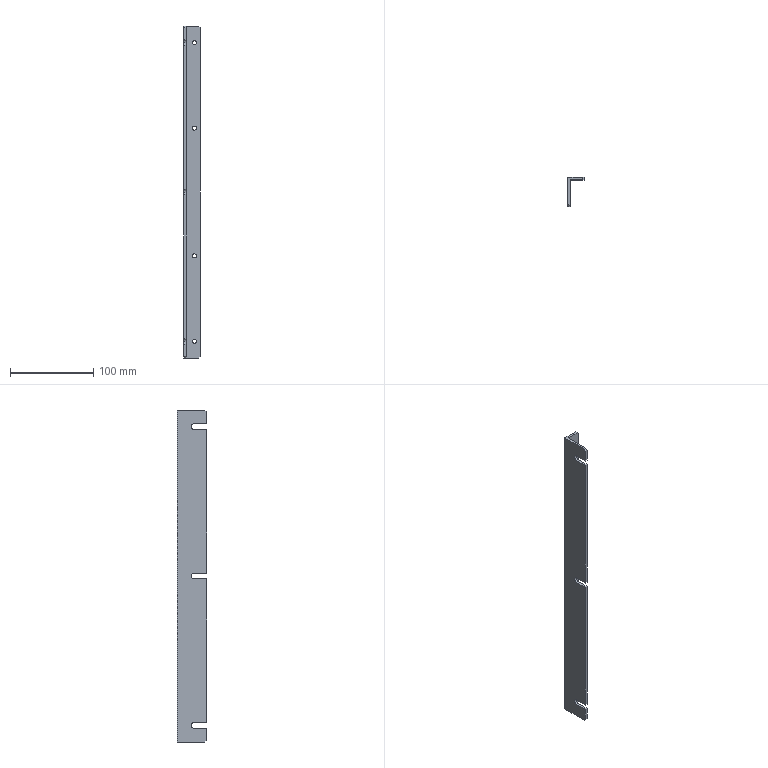Part | SolidWorks | features BaseBody 1 | 1 solid | 35 faces | box 20 x 35 x 400 mm | volume 61095 mm3 | plane 21 | cylinder 14 | commonest cylinder face diameters 5 x8 6.6 x6
STEP:
#1=CARTESIAN_POINT('',(13.,32.,377.5));
#2=VERTEX_POINT('',#1);
#3=CARTESIAN_POINT('',(13.,32.,382.5));
#4=VERTEX_POINT('',#3);
#5=CARTESIAN_POINT('',(13.,32.,380.));
#6=DIRECTION('',(0.,1.,0.));
#7=DIRECTION('',(0.,0.,1.));
#8=AXIS2_PLACEMENT_3D('',#5,#6,#7);
#9=CIRCLE('',#8,2.5);
#10=EDGE_CURVE('',#2,#4,#9,.T.);
#11=ORIENTED_EDGE('',*,*,#10,.F.);
#12=CARTESIAN_POINT('',(13.,35.,377.5));
#13=VERTEX_POINT('',#12);
#14=CARTESIAN_POINT('',(13.,35.,377.5));
#15=DIRECTION('',(0.,1.,0.));
#16=VECTOR('',#15,1000.);
#17=LINE('',#14,#16);
#18=EDGE_CURVE('',#2,#13,#17,.T.);
#19=ORIENTED_EDGE('',*,*,#18,.T.);
#20=CARTESIAN_POINT('',(13.,35.,382.5));
#21=VERTEX_POINT('',#20);
#22=CARTESIAN_POINT('',(13.,35.,380.));
#23=DIRECTION('',(0.,1.,0.));
#24=DIRECTION('',(0.,0.,1.));
#25=AXIS2_PLACEMENT_3D('',#22,#23,#24);
#26=CIRCLE('',#25,2.5);
#27=EDGE_CURVE('',#13,#21,#26,.T.);
#28=ORIENTED_EDGE('',*,*,#27,.T.);
#29=CARTESIAN_POINT('',(13.,35.,382.5));
#30=DIRECTION('',(0.,1.,0.));
#31=VECTOR('',#30,1000.);
#32=LINE('',#29,#31);
#33=EDGE_CURVE('',#4,#21,#32,.T.);
#34=ORIENTED_EDGE('',*,*,#33,.F.);
#35=EDGE_LOOP('',(#11,#19,#28,#34));
#36=FACE_OUTER_BOUND('',#35,.T.);
#37=CARTESIAN_POINT('',(13.,35.,380.));
#38=DIRECTION('',(0.,1.,0.));
#39=DIRECTION('',(0.,0.,1.));
#40=AXIS2_PLACEMENT_3D('',#37,#38,#39);
#41=CYLINDRICAL_SURFACE('',#40,2.5);
#42=ADVANCED_FACE('',(#36),#41,.F.);
#43=CARTESIAN_POINT('',(13.,32.,274.5));
#44=VERTEX_POINT('',#43);
#45=CARTESIAN_POINT('',(13.,32.,279.5));
#46=VERTEX_POINT('',#45);
#47=CARTESIAN_POINT('',(13.,32.,277.));
#48=DIRECTION('',(0.,1.,0.));
#49=DIRECTION('',(0.,0.,1.));
#50=AXIS2_PLACEMENT_3D('',#47,#48,#49);
#51=CIRCLE('',#50,2.5);
#52=EDGE_CURVE('',#44,#46,#51,.T.);
#53=ORIENTED_EDGE('',*,*,#52,.F.);
#54=CARTESIAN_POINT('',(13.,35.,274.5));
#55=VERTEX_POINT('',#54);
#56=CARTESIAN_POINT('',(13.,35.,274.5));
#57=DIRECTION('',(0.,1.,0.));
#58=VECTOR('',#57,1000.);
#59=LINE('',#56,#58);
#60=EDGE_CURVE('',#44,#55,#59,.T.);
#61=ORIENTED_EDGE('',*,*,#60,.T.);
#62=CARTESIAN_POINT('',(13.,35.,279.5));
#63=VERTEX_POINT('',#62);
#64=CARTESIAN_POINT('',(13.,35.,277.));
#65=DIRECTION('',(0.,1.,0.));
#66=DIRECTION('',(0.,0.,1.));
#67=AXIS2_PLACEMENT_3D('',#64,#65,#66);
#68=CIRCLE('',#67,2.5);
#69=EDGE_CURVE('',#55,#63,#68,.T.);
#70=ORIENTED_EDGE('',*,*,#69,.T.);
#71=CARTESIAN_POINT('',(13.,35.,279.5));
#72=DIRECTION('',(0.,1.,0.));
#73=VECTOR('',#72,1000.);
#74=LINE('',#71,#73);
#75=EDGE_CURVE('',#46,#63,#74,.T.);
#76=ORIENTED_EDGE('',*,*,#75,.F.);
#77=EDGE_LOOP('',(#53,#61,#70,#76));
#78=FACE_OUTER_BOUND('',#77,.T.);
#79=CARTESIAN_POINT('',(13.,35.,277.));
#80=DIRECTION('',(0.,1.,0.));
#81=DIRECTION('',(0.,0.,1.));
#82=AXIS2_PLACEMENT_3D('',#79,#80,#81);
#83=CYLINDRICAL_SURFACE('',#82,2.5);
#84=ADVANCED_FACE('',(#78),#83,.F.);
#85=CARTESIAN_POINT('',(13.,32.,120.5));
#86=VERTEX_POINT('',#85);
#87=CARTESIAN_POINT('',(13.,32.,125.5));
#88=VERTEX_POINT('',#87);
#89=CARTESIAN_POINT('',(13.,32.,123.));
#90=DIRECTION('',(0.,1.,0.));
#91=DIRECTION('',(0.,0.,1.));
#92=AXIS2_PLACEMENT_3D('',#89,#90,#91);
#93=CIRCLE('',#92,2.5);
#94=EDGE_CURVE('',#86,#88,#93,.T.);
#95=ORIENTED_EDGE('',*,*,#94,.F.);
#96=CARTESIAN_POINT('',(13.,35.,120.5));
#97=VERTEX_POINT('',#96);
#98=CARTESIAN_POINT('',(13.,35.,120.5));
#99=DIRECTION('',(0.,1.,0.));
#100=VECTOR('',#99,1000.);
#101=LINE('',#98,#100);
#102=EDGE_CURVE('',#86,#97,#101,.T.);
#103=ORIENTED_EDGE('',*,*,#102,.T.);
#104=CARTESIAN_POINT('',(13.,35.,125.5));
#105=VERTEX_POINT('',#104);
#106=CARTESIAN_POINT('',(13.,35.,123.));
#107=DIRECTION('',(0.,1.,0.));
#108=DIRECTION('',(0.,0.,1.));
#109=AXIS2_PLACEMENT_3D('',#106,#107,#108);
#110=CIRCLE('',#109,2.5);
#111=EDGE_CURVE('',#97,#105,#110,.T.);
#112=ORIENTED_EDGE('',*,*,#111,.T.);
#113=CARTESIAN_POINT('',(13.,35.,125.5));
#114=DIRECTION('',(0.,1.,0.));
#115=VECTOR('',#114,1000.);
#116=LINE('',#113,#115);
#117=EDGE_CURVE('',#88,#105,#116,.T.);
#118=ORIENTED_EDGE('',*,*,#117,.F.);
#119=EDGE_LOOP('',(#95,#103,#112,#118));
#120=FACE_OUTER_BOUND('',#119,.T.);
#121=CARTESIAN_POINT('',(13.,35.,123.));
#122=DIRECTION('',(0.,1.,0.));
#123=DIRECTION('',(0.,0.,1.));
#124=AXIS2_PLACEMENT_3D('',#121,#122,#123);
#125=CYLINDRICAL_SURFACE('',#124,2.5);
#126=ADVANCED_FACE('',(#120),#125,.F.);
#127=CARTESIAN_POINT('',(13.,32.,17.5));
#128=VERTEX_POINT('',#127);
#129=CARTESIAN_POINT('',(13.,32.,22.5));
#130=VERTEX_POINT('',#129);
#131=CARTESIAN_POINT('',(13.,32.,20.));
#132=DIRECTION('',(0.,1.,0.));
#133=DIRECTION('',(0.,0.,1.));
#134=AXIS2_PLACEMENT_3D('',#131,#132,#133);
#135=CIRCLE('',#134,2.5);
#136=EDGE_CURVE('',#128,#130,#135,.T.);
#137=ORIENTED_EDGE('',*,*,#136,.F.);
#138=CARTESIAN_POINT('',(13.,35.,17.5));
#139=VERTEX_POINT('',#138);
#140=CARTESIAN_POINT('',(13.,35.,17.5));
#141=DIRECTION('',(0.,1.,0.));
#142=VECTOR('',#141,1000.);
#143=LINE('',#140,#142);
#144=EDGE_CURVE('',#128,#139,#143,.T.);
#145=ORIENTED_EDGE('',*,*,#144,.T.);
#146=CARTESIAN_POINT('',(13.,35.,22.5));
#147=VERTEX_POINT('',#146);
#148=CARTESIAN_POINT('',(13.,35.,20.));
#149=DIRECTION('',(0.,1.,0.));
#150=DIRECTION('',(0.,0.,1.));
#151=AXIS2_PLACEMENT_3D('',#148,#149,#150);
#152=CIRCLE('',#151,2.5);
#153=EDGE_CURVE('',#139,#147,#152,.T.);
#154=ORIENTED_EDGE('',*,*,#153,.T.);
#155=CARTESIAN_POINT('',(13.,35.,22.5));
#156=DIRECTION('',(0.,1.,0.));
#157=VECTOR('',#156,1000.);
#158=LINE('',#155,#157);
#159=EDGE_CURVE('',#130,#147,#158,.T.);
#160=ORIENTED_EDGE('',*,*,#159,.F.);
#161=EDGE_LOOP('',(#137,#145,#154,#160));
#162=FACE_OUTER_BOUND('',#161,.T.);
#163=CARTESIAN_POINT('',(13.,35.,20.));
#164=DIRECTION('',(0.,1.,0.));
#165=DIRECTION('',(0.,0.,1.));
#166=AXIS2_PLACEMENT_3D('',#163,#164,#165);
#167=CYLINDRICAL_SURFACE('',#166,2.5);
#168=ADVANCED_FACE('',(#162),#167,.F.);
#169=CARTESIAN_POINT('',(0.,18.3,20.));
#170=VERTEX_POINT('',#169);
#171=CARTESIAN_POINT('',(0.,15.,23.3));
#172=VERTEX_POINT('',#171);
#173=CARTESIAN_POINT('',(0.,15.,20.));
#174=DIRECTION('',(1.,0.,0.));
#175=DIRECTION('',(0.,1.,0.));
#176=AXIS2_PLACEMENT_3D('',#173,#174,#175);
#177=CIRCLE('',#176,3.3);
#178=EDGE_CURVE('',#170,#172,#177,.T.);
#179=ORIENTED_EDGE('',*,*,#178,.F.);
#180=CARTESIAN_POINT('',(3.,18.3,20.));
#181=VERTEX_POINT('',#180);
#182=CARTESIAN_POINT('',(0.,18.3,20.));
#183=DIRECTION('',(1.,0.,0.));
#184=VECTOR('',#183,1000.);
#185=LINE('',#182,#184);
#186=EDGE_CURVE('',#170,#181,#185,.T.);
#187=ORIENTED_EDGE('',*,*,#186,.T.);
#188=CARTESIAN_POINT('',(3.,15.,23.3));
#189=VERTEX_POINT('',#188);
#190=CARTESIAN_POINT('',(3.,15.,20.));
#191=DIRECTION('',(1.,0.,0.));
#192=DIRECTION('',(0.,1.,0.));
#193=AXIS2_PLACEMENT_3D('',#190,#191,#192);
#194=CIRCLE('',#193,3.3);
#195=EDGE_CURVE('',#181,#189,#194,.T.);
#196=ORIENTED_EDGE('',*,*,#195,.T.);
#197=CARTESIAN_POINT('',(0.,15.,23.3));
#198=DIRECTION('',(1.,0.,0.));
#199=VECTOR('',#198,1000.);
#200=LINE('',#197,#199);
#201=EDGE_CURVE('',#172,#189,#200,.T.);
#202=ORIENTED_EDGE('',*,*,#201,.F.);
#203=EDGE_LOOP('',(#179,#187,#196,#202));
#204=FACE_OUTER_BOUND('',#203,.T.);
#205=CARTESIAN_POINT('',(0.,15.,20.));
#206=DIRECTION('',(1.,0.,0.));
#207=DIRECTION('',(0.,1.,0.));
#208=AXIS2_PLACEMENT_3D('',#205,#206,#207);
#209=CYLINDRICAL_SURFACE('',#208,3.3);
#210=ADVANCED_FACE('',(#204),#209,.F.);
#211=CARTESIAN_POINT('',(0.,18.3,380.));
#212=VERTEX_POINT('',#211);
#213=CARTESIAN_POINT('',(0.,15.,383.3));
#214=VERTEX_POINT('',#213);
#215=CARTESIAN_POINT('',(0.,15.,380.));
#216=DIRECTION('',(1.,0.,0.));
#217=DIRECTION('',(0.,1.,0.));
#218=AXIS2_PLACEMENT_3D('',#215,#216,#217);
#219=CIRCLE('',#218,3.3);
#220=EDGE_CURVE('',#212,#214,#219,.T.);
#221=ORIENTED_EDGE('',*,*,#220,.F.);
#222=CARTESIAN_POINT('',(3.,18.3,380.));
#223=VERTEX_POINT('',#222);
#224=CARTESIAN_POINT('',(0.,18.3,380.));
#225=DIRECTION('',(1.,0.,0.));
#226=VECTOR('',#225,1000.);
#227=LINE('',#224,#226);
#228=EDGE_CURVE('',#212,#223,#227,.T.);
#229=ORIENTED_EDGE('',*,*,#228,.T.);
#230=CARTESIAN_POINT('',(3.,15.,383.3));
#231=VERTEX_POINT('',#230);
#232=CARTESIAN_POINT('',(3.,15.,380.));
#233=DIRECTION('',(1.,0.,0.));
#234=DIRECTION('',(0.,1.,0.));
#235=AXIS2_PLACEMENT_3D('',#232,#233,#234);
#236=CIRCLE('',#235,3.3);
#237=EDGE_CURVE('',#223,#231,#236,.T.);
#238=ORIENTED_EDGE('',*,*,#237,.T.);
#239=CARTESIAN_POINT('',(0.,15.,383.3));
#240=DIRECTION('',(1.,0.,0.));
#241=VECTOR('',#240,1000.);
#242=LINE('',#239,#241);
#243=EDGE_CURVE('',#214,#231,#242,.T.);
#244=ORIENTED_EDGE('',*,*,#243,.F.);
#245=EDGE_LOOP('',(#221,#229,#238,#244));
#246=FACE_OUTER_BOUND('',#245,.T.);
#247=CARTESIAN_POINT('',(0.,15.,380.));
#248=DIRECTION('',(1.,0.,0.));
#249=DIRECTION('',(0.,1.,0.));
#250=AXIS2_PLACEMENT_3D('',#247,#248,#249);
#251=CYLINDRICAL_SURFACE('',#250,3.3);
#252=ADVANCED_FACE('',(#246),#251,.F.);
#253=CARTESIAN_POINT('',(0.,18.3,200.));
#254=VERTEX_POINT('',#253);
#255=CARTESIAN_POINT('',(0.,15.,203.3));
#256=VERTEX_POINT('',#255);
#257=CARTESIAN_POINT('',(0.,15.,200.));
#258=DIRECTION('',(1.,0.,0.));
#259=DIRECTION('',(0.,1.,0.));
#260=AXIS2_PLACEMENT_3D('',#257,#258,#259);
#261=CIRCLE('',#260,3.3);
#262=EDGE_CURVE('',#254,#256,#261,.T.);
#263=ORIENTED_EDGE('',*,*,#262,.F.);
#264=CARTESIAN_POINT('',(3.,18.3,200.));
#265=VERTEX_POINT('',#264);
#266=CARTESIAN_POINT('',(0.,18.3,200.));
#267=DIRECTION('',(1.,0.,0.));
#268=VECTOR('',#267,1000.);
#269=LINE('',#266,#268);
#270=EDGE_CURVE('',#254,#265,#269,.T.);
#271=ORIENTED_EDGE('',*,*,#270,.T.);
#272=CARTESIAN_POINT('',(3.,15.,203.3));
#273=VERTEX_POINT('',#272);
#274=CARTESIAN_POINT('',(3.,15.,200.));
#275=DIRECTION('',(1.,0.,0.));
#276=DIRECTION('',(0.,1.,0.));
#277=AXIS2_PLACEMENT_3D('',#274,#275,#276);
#278=CIRCLE('',#277,3.3);
#279=EDGE_CURVE('',#265,#273,#278,.T.);
#280=ORIENTED_EDGE('',*,*,#279,.T.);
#281=CARTESIAN_POINT('',(0.,15.,203.3));
#282=DIRECTION('',(1.,0.,0.));
#283=VECTOR('',#282,1000.);
#284=LINE('',#281,#283);
#285=EDGE_CURVE('',#256,#273,#284,.T.);
#286=ORIENTED_EDGE('',*,*,#285,.F.);
#287=EDGE_LOOP('',(#263,#271,#280,#286));
#288=FACE_OUTER_BOUND('',#287,.T.);
#289=CARTESIAN_POINT('',(0.,15.,200.));
#290=DIRECTION('',(1.,0.,0.));
#291=DIRECTION('',(0.,1.,0.));
#292=AXIS2_PLACEMENT_3D('',#289,#290,#291);
#293=CYLINDRICAL_SURFACE('',#292,3.3);
#294=ADVANCED_FACE('',(#288),#293,.F.);
#295=CARTESIAN_POINT('',(3.,0.,16.7));
#296=VERTEX_POINT('',#295);
#297=CARTESIAN_POINT('',(3.,15.,16.7));
#298=VERTEX_POINT('',#297);
#299=CARTESIAN_POINT('',(3.,0.,16.7));
#300=DIRECTION('',(0.,1.,0.));
#301=VECTOR('',#300,1000.);
#302=LINE('',#299,#301);
#303=EDGE_CURVE('',#296,#298,#302,.T.);
#304=ORIENTED_EDGE('',*,*,#303,.T.);
#305=CARTESIAN_POINT('',(0.,15.,16.7));
#306=VERTEX_POINT('',#305);
#307=CARTESIAN_POINT('',(0.,15.,16.7));
#308=DIRECTION('',(1.,0.,0.));
#309=VECTOR('',#308,1000.);
#310=LINE('',#307,#309);
#311=EDGE_CURVE('',#306,#298,#310,.T.);
#312=ORIENTED_EDGE('',*,*,#311,.F.);
#313=CARTESIAN_POINT('',(0.,0.,16.7));
#314=VERTEX_POINT('',#313);
#315=CARTESIAN_POINT('',(0.,0.,16.7));
#316=DIRECTION('',(0.,1.,0.));
#317=VECTOR('',#316,1000.);
#318=LINE('',#315,#317);
#319=EDGE_CURVE('',#314,#306,#318,.T.);
#320=ORIENTED_EDGE('',*,*,#319,.F.);
#321=CARTESIAN_POINT('',(0.,0.,16.7));
#322=DIRECTION('',(1.,0.,0.));
#323=VECTOR('',#322,1000.);
#324=LINE('',#321,#323);
#325=EDGE_CURVE('',#314,#296,#324,.T.);
#326=ORIENTED_EDGE('',*,*,#325,.T.);
#327=EDGE_LOOP('',(#304,#312,#320,#326));
#328=FACE_OUTER_BOUND('',#327,.T.);
#329=CARTESIAN_POINT('',(0.,0.,16.7));
#330=DIRECTION('',(0.,0.,-1.));
#331=DIRECTION('',(0.,-1.,0.));
#332=AXIS2_PLACEMENT_3D('',#329,#330,#331);
#333=PLANE('',#332);
#334=ADVANCED_FACE('',(#328),#333,.F.);
#335=CARTESIAN_POINT('',(3.,0.,23.3));
#336=VERTEX_POINT('',#335);
#337=CARTESIAN_POINT('',(3.,0.,23.3));
#338=DIRECTION('',(0.,-1.,0.));
#339=VECTOR('',#338,1000.);
#340=LINE('',#337,#339);
#341=EDGE_CURVE('',#189,#336,#340,.T.);
#342=ORIENTED_EDGE('',*,*,#341,.T.);
#343=CARTESIAN_POINT('',(0.,0.,23.3));
#344=VERTEX_POINT('',#343);
#345=CARTESIAN_POINT('',(0.,0.,23.3));
#346=DIRECTION('',(1.,0.,0.));
#347=VECTOR('',#346,1000.);
#348=LINE('',#345,#347);
#349=EDGE_CURVE('',#344,#336,#348,.T.);
#350=ORIENTED_EDGE('',*,*,#349,.F.);
#351=CARTESIAN_POINT('',(0.,0.,23.3));
#352=DIRECTION('',(0.,-1.,0.));
#353=VECTOR('',#352,1000.);
#354=LINE('',#351,#353);
#355=EDGE_CURVE('',#172,#344,#354,.T.);
#356=ORIENTED_EDGE('',*,*,#355,.F.);
#357=ORIENTED_EDGE('',*,*,#201,.T.);
#358=EDGE_LOOP('',(#342,#350,#356,#357));
#359=FACE_OUTER_BOUND('',#358,.T.);
#360=CARTESIAN_POINT('',(0.,0.,23.3));
#361=DIRECTION('',(0.,0.,1.));
#362=DIRECTION('',(0.,-1.,0.));
#363=AXIS2_PLACEMENT_3D('',#360,#361,#362);
#364=PLANE('',#363);
#365=ADVANCED_FACE('',(#359),#364,.F.);
#366=CARTESIAN_POINT('',(3.,0.,376.7));
#367=VERTEX_POINT('',#366);
#368=CARTESIAN_POINT('',(3.,15.,376.7));
#369=VERTEX_POINT('',#368);
#370=CARTESIAN_POINT('',(3.,0.,376.7));
#371=DIRECTION('',(0.,1.,0.));
#372=VECTOR('',#371,1000.);
#373=LINE('',#370,#372);
#374=EDGE_CURVE('',#367,#369,#373,.T.);
#375=ORIENTED_EDGE('',*,*,#374,.T.);
#376=CARTESIAN_POINT('',(0.,15.,376.7));
#377=VERTEX_POINT('',#376);
#378=CARTESIAN_POINT('',(0.,15.,376.7));
#379=DIRECTION('',(1.,0.,0.));
#380=VECTOR('',#379,1000.);
#381=LINE('',#378,#380);
#382=EDGE_CURVE('',#377,#369,#381,.T.);
#383=ORIENTED_EDGE('',*,*,#382,.F.);
#384=CARTESIAN_POINT('',(0.,0.,376.7));
#385=VERTEX_POINT('',#384);
#386=CARTESIAN_POINT('',(0.,0.,376.7));
#387=DIRECTION('',(0.,1.,0.));
#388=VECTOR('',#387,1000.);
#389=LINE('',#386,#388);
#390=EDGE_CURVE('',#385,#377,#389,.T.);
#391=ORIENTED_EDGE('',*,*,#390,.F.);
#392=CARTESIAN_POINT('',(0.,0.,376.7));
#393=DIRECTION('',(1.,0.,0.));
#394=VECTOR('',#393,1000.);
#395=LINE('',#392,#394);
#396=EDGE_CURVE('',#385,#367,#395,.T.);
#397=ORIENTED_EDGE('',*,*,#396,.T.);
#398=EDGE_LOOP('',(#375,#383,#391,#397));
#399=FACE_OUTER_BOUND('',#398,.T.);
#400=CARTESIAN_POINT('',(0.,0.,376.7));
#401=DIRECTION('',(0.,0.,-1.));
#402=DIRECTION('',(0.,-1.,0.));
#403=AXIS2_PLACEMENT_3D('',#400,#401,#402);
#404=PLANE('',#403);
#405=ADVANCED_FACE('',(#399),#404,.F.);
#406=CARTESIAN_POINT('',(3.,0.,383.3));
#407=VERTEX_POINT('',#406);
#408=CARTESIAN_POINT('',(3.,0.,383.3));
#409=DIRECTION('',(0.,-1.,0.));
#410=VECTOR('',#409,1000.);
#411=LINE('',#408,#410);
#412=EDGE_CURVE('',#231,#407,#411,.T.);
#413=ORIENTED_EDGE('',*,*,#412,.T.);
#414=CARTESIAN_POINT('',(0.,0.,383.3));
#415=VERTEX_POINT('',#414);
#416=CARTESIAN_POINT('',(0.,0.,383.3));
#417=DIRECTION('',(1.,0.,0.));
#418=VECTOR('',#417,1000.);
#419=LINE('',#416,#418);
#420=EDGE_CURVE('',#415,#407,#419,.T.);
#421=ORIENTED_EDGE('',*,*,#420,.F.);
#422=CARTESIAN_POINT('',(0.,0.,383.3));
#423=DIRECTION('',(0.,-1.,0.));
#424=VECTOR('',#423,1000.);
#425=LINE('',#422,#424);
#426=EDGE_CURVE('',#214,#415,#425,.T.);
#427=ORIENTED_EDGE('',*,*,#426,.F.);
#428=ORIENTED_EDGE('',*,*,#243,.T.);
#429=EDGE_LOOP('',(#413,#421,#427,#428));
#430=FACE_OUTER_BOUND('',#429,.T.);
#431=CARTESIAN_POINT('',(0.,0.,383.3));
#432=DIRECTION('',(0.,0.,1.));
#433=DIRECTION('',(1.,0.,0.));
#434=AXIS2_PLACEMENT_3D('',#431,#432,#433);
#435=PLANE('',#434);
#436=ADVANCED_FACE('',(#430),#435,.F.);
#437=CARTESIAN_POINT('',(3.,0.,203.3));
#438=VERTEX_POINT('',#437);
#439=CARTESIAN_POINT('',(3.,15.,203.3));
#440=DIRECTION('',(0.,-1.,0.));
#441=VECTOR('',#440,1000.);
#442=LINE('',#439,#441);
#443=EDGE_CURVE('',#273,#438,#442,.T.);
#444=ORIENTED_EDGE('',*,*,#443,.T.);
#445=CARTESIAN_POINT('',(0.,0.,203.3));
#446=VERTEX_POINT('',#445);
#447=CARTESIAN_POINT('',(0.,0.,203.3));
#448=DIRECTION('',(1.,0.,0.));
#449=VECTOR('',#448,1000.);
#450=LINE('',#447,#449);
#451=EDGE_CURVE('',#446,#438,#450,.T.);
#452=ORIENTED_EDGE('',*,*,#451,.F.);
#453=CARTESIAN_POINT('',(0.,15.,203.3));
#454=DIRECTION('',(0.,-1.,0.));
#455=VECTOR('',#454,1000.);
#456=LINE('',#453,#455);
#457=EDGE_CURVE('',#256,#446,#456,.T.);
#458=ORIENTED_EDGE('',*,*,#457,.F.);
#459=ORIENTED_EDGE('',*,*,#285,.T.);
#460=EDGE_LOOP('',(#444,#452,#458,#459));
#461=FACE_OUTER_BOUND('',#460,.T.);
#462=CARTESIAN_POINT('',(0.,15.,203.3));
#463=DIRECTION('',(0.,0.,1.));
#464=DIRECTION('',(1.,0.,0.));
#465=AXIS2_PLACEMENT_3D('',#462,#463,#464);
#466=PLANE('',#465);
#467=ADVANCED_FACE('',(#461),#466,.F.);
#468=CARTESIAN_POINT('',(3.,0.,196.7));
#469=VERTEX_POINT('',#468);
#470=CARTESIAN_POINT('',(3.,15.,196.7));
#471=VERTEX_POINT('',#470);
#472=CARTESIAN_POINT('',(3.,15.,196.7));
#473=DIRECTION('',(0.,1.,0.));
#474=VECTOR('',#473,1000.);
#475=LINE('',#472,#474);
#476=EDGE_CURVE('',#469,#471,#475,.T.);
#477=ORIENTED_EDGE('',*,*,#476,.T.);
#478=CARTESIAN_POINT('',(0.,15.,196.7));
#479=VERTEX_POINT('',#478);
#480=CARTESIAN_POINT('',(0.,15.,196.7));
#481=DIRECTION('',(1.,0.,0.));
#482=VECTOR('',#481,1000.);
#483=LINE('',#480,#482);
#484=EDGE_CURVE('',#479,#471,#483,.T.);
#485=ORIENTED_EDGE('',*,*,#484,.F.);
#486=CARTESIAN_POINT('',(0.,0.,196.7));
#487=VERTEX_POINT('',#486);
#488=CARTESIAN_POINT('',(0.,15.,196.7));
#489=DIRECTION('',(0.,1.,0.));
#490=VECTOR('',#489,1000.);
#491=LINE('',#488,#490);
#492=EDGE_CURVE('',#487,#479,#491,.T.);
#493=ORIENTED_EDGE('',*,*,#492,.F.);
#494=CARTESIAN_POINT('',(0.,0.,196.7));
#495=DIRECTION('',(1.,0.,0.));
#496=VECTOR('',#495,1000.);
#497=LINE('',#494,#496);
#498=EDGE_CURVE('',#487,#469,#497,.T.);
#499=ORIENTED_EDGE('',*,*,#498,.T.);
#500=EDGE_LOOP('',(#477,#485,#493,#499));
#501=FACE_OUTER_BOUND('',#500,.T.);
#502=CARTESIAN_POINT('',(0.,15.,196.7));
#503=DIRECTION('',(0.,0.,-1.));
#504=DIRECTION('',(0.,-1.,0.));
#505=AXIS2_PLACEMENT_3D('',#502,#503,#504);
#506=PLANE('',#505);
#507=ADVANCED_FACE('',(#501),#506,.F.);
#508=CARTESIAN_POINT('',(20.,32.,398.));
#509=VERTEX_POINT('',#508);
#510=CARTESIAN_POINT('',(18.,32.,400.));
#511=VERTEX_POINT('',#510);
#512=CARTESIAN_POINT('',(18.,32.,400.));
#513=DIRECTION('',(-0.7071,0.,0.7071));
#514=VECTOR('',#513,1000.);
#515=LINE('',#512,#514);
#516=EDGE_CURVE('',#509,#511,#515,.T.);
#517=ORIENTED_EDGE('',*,*,#516,.F.);
#518=CARTESIAN_POINT('',(20.,35.,398.));
#519=VERTEX_POINT('',#518);
#520=CARTESIAN_POINT('',(20.,35.,398.));
#521=DIRECTION('',(0.,-1.,0.));
#522=VECTOR('',#521,1000.);
#523=LINE('',#520,#522);
#524=EDGE_CURVE('',#519,#509,#523,.T.);
#525=ORIENTED_EDGE('',*,*,#524,.F.);
#526=CARTESIAN_POINT('',(18.,35.,400.));
#527=VERTEX_POINT('',#526);
#528=CARTESIAN_POINT('',(18.,35.,400.));
#529=DIRECTION('',(0.7071,0.,-0.7071));
#530=VECTOR('',#529,1000.);
#531=LINE('',#528,#530);
#532=EDGE_CURVE('',#527,#519,#531,.T.);
#533=ORIENTED_EDGE('',*,*,#532,.F.);
#534=CARTESIAN_POINT('',(18.,0.,400.));
#535=DIRECTION('',(0.,1.,0.));
#536=VECTOR('',#535,1000.);
#537=LINE('',#534,#536);
#538=EDGE_CURVE('',#511,#527,#537,.T.);
#539=ORIENTED_EDGE('',*,*,#538,.F.);
#540=EDGE_LOOP('',(#517,#525,#533,#539));
#541=FACE_OUTER_BOUND('',#540,.T.);
#542=CARTESIAN_POINT('',(18.,0.,400.));
#543=DIRECTION('',(-0.7071,0.,-0.7071));
#544=DIRECTION('',(-0.7071,0.,0.7071));
#545=AXIS2_PLACEMENT_3D('',#542,#543,#544);
#546=PLANE('',#545);
#547=ADVANCED_FACE('',(#541),#546,.F.);
#548=CARTESIAN_POINT('',(0.,0.,398.));
#549=VERTEX_POINT('',#548);
#550=CARTESIAN_POINT('',(0.,2.,400.));
#551=VERTEX_POINT('',#550);
#552=CARTESIAN_POINT('',(0.,2.,400.));
#553=DIRECTION('',(0.,0.7071,0.7071));
#554=VECTOR('',#553,1000.);
#555=LINE('',#552,#554);
#556=EDGE_CURVE('',#549,#551,#555,.T.);
#557=ORIENTED_EDGE('',*,*,#556,.F.);
#558=CARTESIAN_POINT('',(3.,0.,398.));
#559=VERTEX_POINT('',#558);
#560=CARTESIAN_POINT('',(3.,0.,398.));
#561=DIRECTION('',(-1.,0.,0.));
#562=VECTOR('',#561,1000.);
#563=LINE('',#560,#562);
#564=EDGE_CURVE('',#559,#549,#563,.T.);
#565=ORIENTED_EDGE('',*,*,#564,.F.);
#566=CARTESIAN_POINT('',(3.,2.,400.));
#567=VERTEX_POINT('',#566);
#568=CARTESIAN_POINT('',(3.,2.,400.));
#569=DIRECTION('',(0.,-0.7071,-0.7071));
#570=VECTOR('',#569,1000.);
#571=LINE('',#568,#570);
#572=EDGE_CURVE('',#567,#559,#571,.T.);
#573=ORIENTED_EDGE('',*,*,#572,.F.);
#574=CARTESIAN_POINT('',(0.,2.,400.));
#575=DIRECTION('',(1.,0.,0.));
#576=VECTOR('',#575,1000.);
#577=LINE('',#574,#576);
#578=EDGE_CURVE('',#551,#567,#577,.T.);
#579=ORIENTED_EDGE('',*,*,#578,.F.);
#580=EDGE_LOOP('',(#557,#565,#573,#579));
#581=FACE_OUTER_BOUND('',#580,.T.);
#582=CARTESIAN_POINT('',(0.,2.,400.));
#583=DIRECTION('',(0.,0.7071,-0.7071));
#584=DIRECTION('',(-1.,0.,0.));
#585=AXIS2_PLACEMENT_3D('',#582,#583,#584);
#586=PLANE('',#585);
#587=ADVANCED_FACE('',(#581),#586,.F.);
#588=CARTESIAN_POINT('',(18.,32.,0.));
#589=VERTEX_POINT('',#588);
#590=CARTESIAN_POINT('',(20.,32.,2.));
#591=VERTEX_POINT('',#590);
#592=CARTESIAN_POINT('',(20.,32.,2.));
#593=DIRECTION('',(0.7071,0.,0.7071));
#594=VECTOR('',#593,1000.);
#595=LINE('',#592,#594);
#596=EDGE_CURVE('',#589,#591,#595,.T.);
#597=ORIENTED_EDGE('',*,*,#596,.F.);
#598=CARTESIAN_POINT('',(18.,35.,0.));
#599=VERTEX_POINT('',#598);
#600=CARTESIAN_POINT('',(18.,32.,0.));
#601=DIRECTION('',(0.,-1.,0.));
#602=VECTOR('',#601,1000.);
#603=LINE('',#600,#602);
#604=EDGE_CURVE('',#599,#589,#603,.T.);
#605=ORIENTED_EDGE('',*,*,#604,.F.);
#606=CARTESIAN_POINT('',(20.,35.,2.));
#607=VERTEX_POINT('',#606);
#608=CARTESIAN_POINT('',(20.,35.,2.));
#609=DIRECTION('',(-0.7071,0.,-0.7071));
#610=VECTOR('',#609,1000.);
#611=LINE('',#608,#610);
#612=EDGE_CURVE('',#607,#599,#611,.T.);
#613=ORIENTED_EDGE('',*,*,#612,.F.);
#614=CARTESIAN_POINT('',(20.,35.,2.));
#615=DIRECTION('',(0.,1.,0.));
#616=VECTOR('',#615,1000.);
#617=LINE('',#614,#616);
#618=EDGE_CURVE('',#591,#607,#617,.T.);
#619=ORIENTED_EDGE('',*,*,#618,.F.);
#620=EDGE_LOOP('',(#597,#605,#613,#619));
#621=FACE_OUTER_BOUND('',#620,.T.);
#622=CARTESIAN_POINT('',(20.,35.,2.));
#623=DIRECTION('',(0.7071,0.,-0.7071));
#624=DIRECTION('',(0.,-1.,0.));
#625=AXIS2_PLACEMENT_3D('',#622,#623,#624);
#626=PLANE('',#625);
#627=ADVANCED_FACE('',(#621),#626,.T.);
#628=CARTESIAN_POINT('',(0.,2.,0.));
#629=VERTEX_POINT('',#628);
#630=CARTESIAN_POINT('',(0.,0.,2.));
#631=VERTEX_POINT('',#630);
#632=CARTESIAN_POINT('',(0.,0.,2.));
#633=DIRECTION('',(0.,-0.7071,0.7071));
#634=VECTOR('',#633,1000.);
#635=LINE('',#632,#634);
#636=EDGE_CURVE('',#629,#631,#635,.T.);
#637=ORIENTED_EDGE('',*,*,#636,.F.);
#638=CARTESIAN_POINT('',(3.,2.,0.));
#639=VERTEX_POINT('',#638);
#640=CARTESIAN_POINT('',(0.,2.,0.));
#641=DIRECTION('',(-1.,0.,0.));
#642=VECTOR('',#641,1000.);
#643=LINE('',#640,#642);
#644=EDGE_CURVE('',#639,#629,#643,.T.);
#645=ORIENTED_EDGE('',*,*,#644,.F.);
#646=CARTESIAN_POINT('',(3.,0.,2.));
#647=VERTEX_POINT('',#646);
#648=CARTESIAN_POINT('',(3.,0.,2.));
#649=DIRECTION('',(0.,0.7071,-0.7071));
#650=VECTOR('',#649,1000.);
#651=LINE('',#648,#650);
#652=EDGE_CURVE('',#647,#639,#651,.T.);
#653=ORIENTED_EDGE('',*,*,#652,.F.);
#654=CARTESIAN_POINT('',(3.,0.,2.));
#655=DIRECTION('',(1.,0.,0.));
#656=VECTOR('',#655,1000.);
#657=LINE('',#654,#656);
#658=EDGE_CURVE('',#631,#647,#657,.T.);
#659=ORIENTED_EDGE('',*,*,#658,.F.);
#660=EDGE_LOOP('',(#637,#645,#653,#659));
#661=FACE_OUTER_BOUND('',#660,.T.);
#662=CARTESIAN_POINT('',(3.,0.,2.));
#663=DIRECTION('',(0.,-0.7071,-0.7071));
#664=DIRECTION('',(0.,-0.7071,0.7071));
#665=AXIS2_PLACEMENT_3D('',#662,#663,#664);
#666=PLANE('',#665);
#667=ADVANCED_FACE('',(#661),#666,.T.);
#668=CARTESIAN_POINT('',(3.,32.,0.));
#669=VERTEX_POINT('',#668);
#670=CARTESIAN_POINT('',(3.,32.,0.));
#671=DIRECTION('',(0.,1.,0.));
#672=VECTOR('',#671,1000.);
#673=LINE('',#670,#672);
#674=EDGE_CURVE('',#639,#669,#673,.T.);
#675=ORIENTED_EDGE('',*,*,#674,.F.);
#676=ORIENTED_EDGE('',*,*,#644,.T.);
#677=CARTESIAN_POINT('',(0.,35.,0.));
#678=VERTEX_POINT('',#677);
#679=CARTESIAN_POINT('',(0.,0.,0.));
#680=DIRECTION('',(0.,-1.,0.));
#681=VECTOR('',#680,1000.);
#682=LINE('',#679,#681);
#683=EDGE_CURVE('',#678,#629,#682,.T.);
#684=ORIENTED_EDGE('',*,*,#683,.F.);
#685=CARTESIAN_POINT('',(0.,35.,0.));
#686=DIRECTION('',(-1.,0.,0.));
#687=VECTOR('',#686,1000.);
#688=LINE('',#685,#687);
#689=EDGE_CURVE('',#599,#678,#688,.T.);
#690=ORIENTED_EDGE('',*,*,#689,.F.);
#691=ORIENTED_EDGE('',*,*,#604,.T.);
#692=CARTESIAN_POINT('',(20.,32.,0.));
#693=DIRECTION('',(1.,0.,0.));
#694=VECTOR('',#693,1000.);
#695=LINE('',#692,#694);
#696=EDGE_CURVE('',#669,#589,#695,.T.);
#697=ORIENTED_EDGE('',*,*,#696,.F.);
#698=EDGE_LOOP('',(#675,#676,#684,#690,#691,#697));
#699=FACE_OUTER_BOUND('',#698,.T.);
#700=CARTESIAN_POINT('',(0.,0.,0.));
#701=DIRECTION('',(0.,0.,-1.));
#702=DIRECTION('',(0.,-1.,0.));
#703=AXIS2_PLACEMENT_3D('',#700,#701,#702);
#704=PLANE('',#703);
#705=ADVANCED_FACE('',(#699),#704,.T.);
#706=CARTESIAN_POINT('',(0.,35.,400.));
#707=VERTEX_POINT('',#706);
#708=CARTESIAN_POINT('',(0.,0.,400.));
#709=DIRECTION('',(0.,-1.,0.));
#710=VECTOR('',#709,1000.);
#711=LINE('',#708,#710);
#712=EDGE_CURVE('',#707,#551,#711,.T.);
#713=ORIENTED_EDGE('',*,*,#712,.T.);
#714=ORIENTED_EDGE('',*,*,#578,.T.);
#715=CARTESIAN_POINT('',(3.,32.,400.));
#716=VERTEX_POINT('',#715);
#717=CARTESIAN_POINT('',(3.,32.,400.));
#718=DIRECTION('',(0.,1.,0.));
#719=VECTOR('',#718,1000.);
#720=LINE('',#717,#719);
#721=EDGE_CURVE('',#567,#716,#720,.T.);
#722=ORIENTED_EDGE('',*,*,#721,.T.);
#723=CARTESIAN_POINT('',(20.,32.,400.));
#724=DIRECTION('',(1.,0.,0.));
#725=VECTOR('',#724,1000.);
#726=LINE('',#723,#725);
#727=EDGE_CURVE('',#716,#511,#726,.T.);
#728=ORIENTED_EDGE('',*,*,#727,.T.);
#729=ORIENTED_EDGE('',*,*,#538,.T.);
#730=CARTESIAN_POINT('',(0.,35.,400.));
#731=DIRECTION('',(-1.,0.,0.));
#732=VECTOR('',#731,1000.);
#733=LINE('',#730,#732);
#734=EDGE_CURVE('',#527,#707,#733,.T.);
#735=ORIENTED_EDGE('',*,*,#734,.T.);
#736=EDGE_LOOP('',(#713,#714,#722,#728,#729,#735));
#737=FACE_OUTER_BOUND('',#736,.T.);
#738=CARTESIAN_POINT('',(0.,0.,400.));
#739=DIRECTION('',(0.,0.,-1.));
#740=DIRECTION('',(0.,-1.,0.));
#741=AXIS2_PLACEMENT_3D('',#738,#739,#740);
#742=PLANE('',#741);
#743=ADVANCED_FACE('',(#737),#742,.F.);
#744=ORIENTED_EDGE('',*,*,#319,.T.);
#745=CARTESIAN_POINT('',(0.,15.,20.));
#746=DIRECTION('',(1.,0.,0.));
#747=DIRECTION('',(0.,1.,0.));
#748=AXIS2_PLACEMENT_3D('',#745,#746,#747);
#749=CIRCLE('',#748,3.3);
#750=EDGE_CURVE('',#306,#170,#749,.T.);
#751=ORIENTED_EDGE('',*,*,#750,.T.);
#752=ORIENTED_EDGE('',*,*,#178,.T.);
#753=ORIENTED_EDGE('',*,*,#355,.T.);
#754=CARTESIAN_POINT('',(0.,0.,400.));
#755=DIRECTION('',(0.,0.,-1.));
#756=VECTOR('',#755,1000.);
#757=LINE('',#754,#756);
#758=EDGE_CURVE('',#487,#344,#757,.T.);
#759=ORIENTED_EDGE('',*,*,#758,.F.);
#760=ORIENTED_EDGE('',*,*,#492,.T.);
#761=CARTESIAN_POINT('',(0.,15.,200.));
#762=DIRECTION('',(1.,0.,0.));
#763=DIRECTION('',(0.,1.,0.));
#764=AXIS2_PLACEMENT_3D('',#761,#762,#763);
#765=CIRCLE('',#764,3.3);
#766=EDGE_CURVE('',#479,#254,#765,.T.);
#767=ORIENTED_EDGE('',*,*,#766,.T.);
#768=ORIENTED_EDGE('',*,*,#262,.T.);
#769=ORIENTED_EDGE('',*,*,#457,.T.);
#770=CARTESIAN_POINT('',(0.,0.,400.));
#771=DIRECTION('',(0.,0.,-1.));
#772=VECTOR('',#771,1000.);
#773=LINE('',#770,#772);
#774=EDGE_CURVE('',#385,#446,#773,.T.);
#775=ORIENTED_EDGE('',*,*,#774,.F.);
#776=ORIENTED_EDGE('',*,*,#390,.T.);
#777=CARTESIAN_POINT('',(0.,15.,380.));
#778=DIRECTION('',(1.,0.,0.));
#779=DIRECTION('',(0.,1.,0.));
#780=AXIS2_PLACEMENT_3D('',#777,#778,#779);
#781=CIRCLE('',#780,3.3);
#782=EDGE_CURVE('',#377,#212,#781,.T.);
#783=ORIENTED_EDGE('',*,*,#782,.T.);
#784=ORIENTED_EDGE('',*,*,#220,.T.);
#785=ORIENTED_EDGE('',*,*,#426,.T.);
#786=CARTESIAN_POINT('',(0.,0.,400.));
#787=DIRECTION('',(0.,0.,-1.));
#788=VECTOR('',#787,1000.);
#789=LINE('',#786,#788);
#790=EDGE_CURVE('',#549,#415,#789,.T.);
#791=ORIENTED_EDGE('',*,*,#790,.F.);
#792=ORIENTED_EDGE('',*,*,#556,.T.);
#793=ORIENTED_EDGE('',*,*,#712,.F.);
#794=CARTESIAN_POINT('',(0.,35.,400.));
#795=DIRECTION('',(0.,0.,-1.));
#796=VECTOR('',#795,1000.);
#797=LINE('',#794,#796);
#798=EDGE_CURVE('',#707,#678,#797,.T.);
#799=ORIENTED_EDGE('',*,*,#798,.T.);
#800=ORIENTED_EDGE('',*,*,#683,.T.);
#801=ORIENTED_EDGE('',*,*,#636,.T.);
#802=CARTESIAN_POINT('',(0.,0.,400.));
#803=DIRECTION('',(0.,0.,-1.));
#804=VECTOR('',#803,1000.);
#805=LINE('',#802,#804);
#806=EDGE_CURVE('',#314,#631,#805,.T.);
#807=ORIENTED_EDGE('',*,*,#806,.F.);
#808=EDGE_LOOP('',(#744,#751,#752,#753,#759,#760,#767,#768,#769,#775,#776,#783,#784,#785,#791,#792,#793,#799,#800,#801,#807));
#809=FACE_OUTER_BOUND('',#808,.T.);
#810=CARTESIAN_POINT('',(0.,0.,400.));
#811=DIRECTION('',(1.,0.,0.));
#812=DIRECTION('',(0.,1.,0.));
#813=AXIS2_PLACEMENT_3D('',#810,#811,#812);
#814=PLANE('',#813);
#815=ADVANCED_FACE('',(#809),#814,.F.);
#816=CARTESIAN_POINT('',(13.,35.,20.));
#817=DIRECTION('',(0.,1.,0.));
#818=DIRECTION('',(0.,0.,1.));
#819=AXIS2_PLACEMENT_3D('',#816,#817,#818);
#820=CIRCLE('',#819,2.5);
#821=EDGE_CURVE('',#147,#139,#820,.T.);
#822=ORIENTED_EDGE('',*,*,#821,.F.);
#823=ORIENTED_EDGE('',*,*,#153,.F.);
#824=EDGE_LOOP('',(#822,#823));
#825=FACE_BOUND('',#824,.T.);
#826=CARTESIAN_POINT('',(13.,35.,123.));
#827=DIRECTION('',(0.,1.,0.));
#828=DIRECTION('',(0.,0.,1.));
#829=AXIS2_PLACEMENT_3D('',#826,#827,#828);
#830=CIRCLE('',#829,2.5);
#831=EDGE_CURVE('',#105,#97,#830,.T.);
#832=ORIENTED_EDGE('',*,*,#831,.F.);
#833=ORIENTED_EDGE('',*,*,#111,.F.);
#834=EDGE_LOOP('',(#832,#833));
#835=FACE_BOUND('',#834,.T.);
#836=CARTESIAN_POINT('',(13.,35.,277.));
#837=DIRECTION('',(0.,1.,0.));
#838=DIRECTION('',(0.,0.,1.));
#839=AXIS2_PLACEMENT_3D('',#836,#837,#838);
#840=CIRCLE('',#839,2.5);
#841=EDGE_CURVE('',#63,#55,#840,.T.);
#842=ORIENTED_EDGE('',*,*,#841,.F.);
#843=ORIENTED_EDGE('',*,*,#69,.F.);
#844=EDGE_LOOP('',(#842,#843));
#845=FACE_BOUND('',#844,.T.);
#846=CARTESIAN_POINT('',(13.,35.,380.));
#847=DIRECTION('',(0.,1.,0.));
#848=DIRECTION('',(0.,0.,1.));
#849=AXIS2_PLACEMENT_3D('',#846,#847,#848);
#850=CIRCLE('',#849,2.5);
#851=EDGE_CURVE('',#21,#13,#850,.T.);
#852=ORIENTED_EDGE('',*,*,#851,.F.);
#853=ORIENTED_EDGE('',*,*,#27,.F.);
#854=EDGE_LOOP('',(#852,#853));
#855=FACE_BOUND('',#854,.T.);
#856=CARTESIAN_POINT('',(20.,35.,400.));
#857=DIRECTION('',(0.,0.,-1.));
#858=VECTOR('',#857,1000.);
#859=LINE('',#856,#858);
#860=EDGE_CURVE('',#519,#607,#859,.T.);
#861=ORIENTED_EDGE('',*,*,#860,.T.);
#862=ORIENTED_EDGE('',*,*,#612,.T.);
#863=ORIENTED_EDGE('',*,*,#689,.T.);
#864=ORIENTED_EDGE('',*,*,#798,.F.);
#865=ORIENTED_EDGE('',*,*,#734,.F.);
#866=ORIENTED_EDGE('',*,*,#532,.T.);
#867=EDGE_LOOP('',(#861,#862,#863,#864,#865,#866));
#868=FACE_OUTER_BOUND('',#867,.T.);
#869=CARTESIAN_POINT('',(0.,35.,400.));
#870=DIRECTION('',(0.,-1.,0.));
#871=DIRECTION('',(0.,0.,-1.));
#872=AXIS2_PLACEMENT_3D('',#869,#870,#871);
#873=PLANE('',#872);
#874=ADVANCED_FACE('',(#825,#835,#845,#855,#868),#873,.F.);
#875=CARTESIAN_POINT('',(20.,32.,400.));
#876=DIRECTION('',(0.,0.,-1.));
#877=VECTOR('',#876,1000.);
#878=LINE('',#875,#877);
#879=EDGE_CURVE('',#509,#591,#878,.T.);
#880=ORIENTED_EDGE('',*,*,#879,.T.);
#881=ORIENTED_EDGE('',*,*,#618,.T.);
#882=ORIENTED_EDGE('',*,*,#860,.F.);
#883=ORIENTED_EDGE('',*,*,#524,.T.);
#884=EDGE_LOOP('',(#880,#881,#882,#883));
#885=FACE_OUTER_BOUND('',#884,.T.);
#886=CARTESIAN_POINT('',(20.,35.,400.));
#887=DIRECTION('',(-1.,0.,0.));
#888=DIRECTION('',(0.,0.,1.));
#889=AXIS2_PLACEMENT_3D('',#886,#887,#888);
#890=PLANE('',#889);
#891=ADVANCED_FACE('',(#885),#890,.F.);
#892=CARTESIAN_POINT('',(13.,32.,20.));
#893=DIRECTION('',(0.,1.,0.));
#894=DIRECTION('',(0.,0.,1.));
#895=AXIS2_PLACEMENT_3D('',#892,#893,#894);
#896=CIRCLE('',#895,2.5);
#897=EDGE_CURVE('',#130,#128,#896,.T.);
#898=ORIENTED_EDGE('',*,*,#897,.T.);
#899=ORIENTED_EDGE('',*,*,#136,.T.);
#900=EDGE_LOOP('',(#898,#899));
#901=FACE_BOUND('',#900,.T.);
#902=CARTESIAN_POINT('',(13.,32.,123.));
#903=DIRECTION('',(0.,1.,0.));
#904=DIRECTION('',(0.,0.,1.));
#905=AXIS2_PLACEMENT_3D('',#902,#903,#904);
#906=CIRCLE('',#905,2.5);
#907=EDGE_CURVE('',#88,#86,#906,.T.);
#908=ORIENTED_EDGE('',*,*,#907,.T.);
#909=ORIENTED_EDGE('',*,*,#94,.T.);
#910=EDGE_LOOP('',(#908,#909));
#911=FACE_BOUND('',#910,.T.);
#912=CARTESIAN_POINT('',(13.,32.,277.));
#913=DIRECTION('',(0.,1.,0.));
#914=DIRECTION('',(0.,0.,1.));
#915=AXIS2_PLACEMENT_3D('',#912,#913,#914);
#916=CIRCLE('',#915,2.5);
#917=EDGE_CURVE('',#46,#44,#916,.T.);
#918=ORIENTED_EDGE('',*,*,#917,.T.);
#919=ORIENTED_EDGE('',*,*,#52,.T.);
#920=EDGE_LOOP('',(#918,#919));
#921=FACE_BOUND('',#920,.T.);
#922=CARTESIAN_POINT('',(13.,32.,380.));
#923=DIRECTION('',(0.,1.,0.));
#924=DIRECTION('',(0.,0.,1.));
#925=AXIS2_PLACEMENT_3D('',#922,#923,#924);
#926=CIRCLE('',#925,2.5);
#927=EDGE_CURVE('',#4,#2,#926,.T.);
#928=ORIENTED_EDGE('',*,*,#927,.T.);
#929=ORIENTED_EDGE('',*,*,#10,.T.);
#930=EDGE_LOOP('',(#928,#929));
#931=FACE_BOUND('',#930,.T.);
#932=ORIENTED_EDGE('',*,*,#696,.T.);
#933=ORIENTED_EDGE('',*,*,#596,.T.);
#934=ORIENTED_EDGE('',*,*,#879,.F.);
#935=ORIENTED_EDGE('',*,*,#516,.T.);
#936=ORIENTED_EDGE('',*,*,#727,.F.);
#937=CARTESIAN_POINT('',(3.,32.,400.));
#938=DIRECTION('',(0.,0.,-1.));
#939=VECTOR('',#938,1000.);
#940=LINE('',#937,#939);
#941=EDGE_CURVE('',#716,#669,#940,.T.);
#942=ORIENTED_EDGE('',*,*,#941,.T.);
#943=EDGE_LOOP('',(#932,#933,#934,#935,#936,#942));
#944=FACE_OUTER_BOUND('',#943,.T.);
#945=CARTESIAN_POINT('',(20.,32.,400.));
#946=DIRECTION('',(0.,1.,0.));
#947=DIRECTION('',(1.,0.,0.));
#948=AXIS2_PLACEMENT_3D('',#945,#946,#947);
#949=PLANE('',#948);
#950=ADVANCED_FACE('',(#901,#911,#921,#931,#944),#949,.F.);
#951=CARTESIAN_POINT('',(3.,0.,400.));
#952=DIRECTION('',(0.,0.,-1.));
#953=VECTOR('',#952,1000.);
#954=LINE('',#951,#953);
#955=EDGE_CURVE('',#469,#336,#954,.T.);
#956=ORIENTED_EDGE('',*,*,#955,.T.);
#957=ORIENTED_EDGE('',*,*,#341,.F.);
#958=ORIENTED_EDGE('',*,*,#195,.F.);
#959=CARTESIAN_POINT('',(3.,15.,20.));
#960=DIRECTION('',(1.,0.,0.));
#961=DIRECTION('',(0.,1.,0.));
#962=AXIS2_PLACEMENT_3D('',#959,#960,#961);
#963=CIRCLE('',#962,3.3);
#964=EDGE_CURVE('',#298,#181,#963,.T.);
#965=ORIENTED_EDGE('',*,*,#964,.F.);
#966=ORIENTED_EDGE('',*,*,#303,.F.);
#967=CARTESIAN_POINT('',(3.,0.,400.));
#968=DIRECTION('',(0.,0.,-1.));
#969=VECTOR('',#968,1000.);
#970=LINE('',#967,#969);
#971=EDGE_CURVE('',#296,#647,#970,.T.);
#972=ORIENTED_EDGE('',*,*,#971,.T.);
#973=ORIENTED_EDGE('',*,*,#652,.T.);
#974=ORIENTED_EDGE('',*,*,#674,.T.);
#975=ORIENTED_EDGE('',*,*,#941,.F.);
#976=ORIENTED_EDGE('',*,*,#721,.F.);
#977=ORIENTED_EDGE('',*,*,#572,.T.);
#978=CARTESIAN_POINT('',(3.,0.,400.));
#979=DIRECTION('',(0.,0.,-1.));
#980=VECTOR('',#979,1000.);
#981=LINE('',#978,#980);
#982=EDGE_CURVE('',#559,#407,#981,.T.);
#983=ORIENTED_EDGE('',*,*,#982,.T.);
#984=ORIENTED_EDGE('',*,*,#412,.F.);
#985=ORIENTED_EDGE('',*,*,#237,.F.);
#986=CARTESIAN_POINT('',(3.,15.,380.));
#987=DIRECTION('',(1.,0.,0.));
#988=DIRECTION('',(0.,1.,0.));
#989=AXIS2_PLACEMENT_3D('',#986,#987,#988);
#990=CIRCLE('',#989,3.3);
#991=EDGE_CURVE('',#369,#223,#990,.T.);
#992=ORIENTED_EDGE('',*,*,#991,.F.);
#993=ORIENTED_EDGE('',*,*,#374,.F.);
#994=CARTESIAN_POINT('',(3.,0.,400.));
#995=DIRECTION('',(0.,0.,-1.));
#996=VECTOR('',#995,1000.);
#997=LINE('',#994,#996);
#998=EDGE_CURVE('',#367,#438,#997,.T.);
#999=ORIENTED_EDGE('',*,*,#998,.T.);
#1000=ORIENTED_EDGE('',*,*,#443,.F.);
#1001=ORIENTED_EDGE('',*,*,#279,.F.);
#1002=CARTESIAN_POINT('',(3.,15.,200.));
#1003=DIRECTION('',(1.,0.,0.));
#1004=DIRECTION('',(0.,1.,0.));
#1005=AXIS2_PLACEMENT_3D('',#1002,#1003,#1004);
#1006=CIRCLE('',#1005,3.3);
#1007=EDGE_CURVE('',#471,#265,#1006,.T.);
#1008=ORIENTED_EDGE('',*,*,#1007,.F.);
#1009=ORIENTED_EDGE('',*,*,#476,.F.);
#1010=EDGE_LOOP('',(#956,#957,#958,#965,#966,#972,#973,#974,#975,#976,#977,#983,#984,#985,#992,#993,#999,#1000,#1001,#1008,#1009));
#1011=FACE_OUTER_BOUND('',#1010,.T.);
#1012=CARTESIAN_POINT('',(3.,32.,400.));
#1013=DIRECTION('',(-1.,0.,0.));
#1014=DIRECTION('',(0.,1.,0.));
#1015=AXIS2_PLACEMENT_3D('',#1012,#1013,#1014);
#1016=PLANE('',#1015);
#1017=ADVANCED_FACE('',(#1011),#1016,.F.);
#1018=ORIENTED_EDGE('',*,*,#998,.F.);
#1019=ORIENTED_EDGE('',*,*,#396,.F.);
#1020=ORIENTED_EDGE('',*,*,#774,.T.);
#1021=ORIENTED_EDGE('',*,*,#451,.T.);
#1022=EDGE_LOOP('',(#1018,#1019,#1020,#1021));
#1023=FACE_OUTER_BOUND('',#1022,.T.);
#1024=CARTESIAN_POINT('',(3.,0.,400.));
#1025=DIRECTION('',(0.,1.,0.));
#1026=DIRECTION('',(1.,0.,0.));
#1027=AXIS2_PLACEMENT_3D('',#1024,#1025,#1026);
#1028=PLANE('',#1027);
#1029=ADVANCED_FACE('',(#1023),#1028,.F.);
#1030=ORIENTED_EDGE('',*,*,#971,.F.);
#1031=ORIENTED_EDGE('',*,*,#325,.F.);
#1032=ORIENTED_EDGE('',*,*,#806,.T.);
#1033=ORIENTED_EDGE('',*,*,#658,.T.);
#1034=EDGE_LOOP('',(#1030,#1031,#1032,#1033));
#1035=FACE_OUTER_BOUND('',#1034,.T.);
#1036=CARTESIAN_POINT('',(3.,0.,400.));
#1037=DIRECTION('',(0.,1.,0.));
#1038=DIRECTION('',(1.,0.,0.));
#1039=AXIS2_PLACEMENT_3D('',#1036,#1037,#1038);
#1040=PLANE('',#1039);
#1041=ADVANCED_FACE('',(#1035),#1040,.F.);
#1042=ORIENTED_EDGE('',*,*,#790,.T.);
#1043=ORIENTED_EDGE('',*,*,#420,.T.);
#1044=ORIENTED_EDGE('',*,*,#982,.F.);
#1045=ORIENTED_EDGE('',*,*,#564,.T.);
#1046=EDGE_LOOP('',(#1042,#1043,#1044,#1045));
#1047=FACE_OUTER_BOUND('',#1046,.T.);
#1048=CARTESIAN_POINT('',(3.,0.,400.));
#1049=DIRECTION('',(0.,1.,0.));
#1050=DIRECTION('',(1.,0.,0.));
#1051=AXIS2_PLACEMENT_3D('',#1048,#1049,#1050);
#1052=PLANE('',#1051);
#1053=ADVANCED_FACE('',(#1047),#1052,.F.);
#1054=ORIENTED_EDGE('',*,*,#758,.T.);
#1055=ORIENTED_EDGE('',*,*,#349,.T.);
#1056=ORIENTED_EDGE('',*,*,#955,.F.);
#1057=ORIENTED_EDGE('',*,*,#498,.F.);
#1058=EDGE_LOOP('',(#1054,#1055,#1056,#1057));
#1059=FACE_OUTER_BOUND('',#1058,.T.);
#1060=CARTESIAN_POINT('',(3.,0.,400.));
#1061=DIRECTION('',(0.,1.,0.));
#1062=DIRECTION('',(1.,0.,0.));
#1063=AXIS2_PLACEMENT_3D('',#1060,#1061,#1062);
#1064=PLANE('',#1063);
#1065=ADVANCED_FACE('',(#1059),#1064,.F.);
#1066=ORIENTED_EDGE('',*,*,#270,.F.);
#1067=ORIENTED_EDGE('',*,*,#766,.F.);
#1068=ORIENTED_EDGE('',*,*,#484,.T.);
#1069=ORIENTED_EDGE('',*,*,#1007,.T.);
#1070=EDGE_LOOP('',(#1066,#1067,#1068,#1069));
#1071=FACE_OUTER_BOUND('',#1070,.T.);
#1072=CARTESIAN_POINT('',(0.,15.,200.));
#1073=DIRECTION('',(1.,0.,0.));
#1074=DIRECTION('',(0.,1.,0.));
#1075=AXIS2_PLACEMENT_3D('',#1072,#1073,#1074);
#1076=CYLINDRICAL_SURFACE('',#1075,3.3);
#1077=ADVANCED_FACE('',(#1071),#1076,.F.);
#1078=ORIENTED_EDGE('',*,*,#228,.F.);
#1079=ORIENTED_EDGE('',*,*,#782,.F.);
#1080=ORIENTED_EDGE('',*,*,#382,.T.);
#1081=ORIENTED_EDGE('',*,*,#991,.T.);
#1082=EDGE_LOOP('',(#1078,#1079,#1080,#1081));
#1083=FACE_OUTER_BOUND('',#1082,.T.);
#1084=CARTESIAN_POINT('',(0.,15.,380.));
#1085=DIRECTION('',(1.,0.,0.));
#1086=DIRECTION('',(0.,1.,0.));
#1087=AXIS2_PLACEMENT_3D('',#1084,#1085,#1086);
#1088=CYLINDRICAL_SURFACE('',#1087,3.3);
#1089=ADVANCED_FACE('',(#1083),#1088,.F.);
#1090=ORIENTED_EDGE('',*,*,#186,.F.);
#1091=ORIENTED_EDGE('',*,*,#750,.F.);
#1092=ORIENTED_EDGE('',*,*,#311,.T.);
#1093=ORIENTED_EDGE('',*,*,#964,.T.);
#1094=EDGE_LOOP('',(#1090,#1091,#1092,#1093));
#1095=FACE_OUTER_BOUND('',#1094,.T.);
#1096=CARTESIAN_POINT('',(0.,15.,20.));
#1097=DIRECTION('',(1.,0.,0.));
#1098=DIRECTION('',(0.,1.,0.));
#1099=AXIS2_PLACEMENT_3D('',#1096,#1097,#1098);
#1100=CYLINDRICAL_SURFACE('',#1099,3.3);
#1101=ADVANCED_FACE('',(#1095),#1100,.F.);
#1102=ORIENTED_EDGE('',*,*,#144,.F.);
#1103=ORIENTED_EDGE('',*,*,#897,.F.);
#1104=ORIENTED_EDGE('',*,*,#159,.T.);
#1105=ORIENTED_EDGE('',*,*,#821,.T.);
#1106=EDGE_LOOP('',(#1102,#1103,#1104,#1105));
#1107=FACE_OUTER_BOUND('',#1106,.T.);
#1108=CARTESIAN_POINT('',(13.,35.,20.));
#1109=DIRECTION('',(0.,1.,0.));
#1110=DIRECTION('',(0.,0.,1.));
#1111=AXIS2_PLACEMENT_3D('',#1108,#1109,#1110);
#1112=CYLINDRICAL_SURFACE('',#1111,2.5);
#1113=ADVANCED_FACE('',(#1107),#1112,.F.);
#1114=ORIENTED_EDGE('',*,*,#102,.F.);
#1115=ORIENTED_EDGE('',*,*,#907,.F.);
#1116=ORIENTED_EDGE('',*,*,#117,.T.);
#1117=ORIENTED_EDGE('',*,*,#831,.T.);
#1118=EDGE_LOOP('',(#1114,#1115,#1116,#1117));
#1119=FACE_OUTER_BOUND('',#1118,.T.);
#1120=CARTESIAN_POINT('',(13.,35.,123.));
#1121=DIRECTION('',(0.,1.,0.));
#1122=DIRECTION('',(0.,0.,1.));
#1123=AXIS2_PLACEMENT_3D('',#1120,#1121,#1122);
#1124=CYLINDRICAL_SURFACE('',#1123,2.5);
#1125=ADVANCED_FACE('',(#1119),#1124,.F.);
#1126=ORIENTED_EDGE('',*,*,#60,.F.);
#1127=ORIENTED_EDGE('',*,*,#917,.F.);
#1128=ORIENTED_EDGE('',*,*,#75,.T.);
#1129=ORIENTED_EDGE('',*,*,#841,.T.);
#1130=EDGE_LOOP('',(#1126,#1127,#1128,#1129));
#1131=FACE_OUTER_BOUND('',#1130,.T.);
#1132=CARTESIAN_POINT('',(13.,35.,277.));
#1133=DIRECTION('',(0.,1.,0.));
#1134=DIRECTION('',(0.,0.,1.));
#1135=AXIS2_PLACEMENT_3D('',#1132,#1133,#1134);
#1136=CYLINDRICAL_SURFACE('',#1135,2.5);
#1137=ADVANCED_FACE('',(#1131),#1136,.F.);
#1138=ORIENTED_EDGE('',*,*,#18,.F.);
#1139=ORIENTED_EDGE('',*,*,#927,.F.);
#1140=ORIENTED_EDGE('',*,*,#33,.T.);
#1141=ORIENTED_EDGE('',*,*,#851,.T.);
#1142=EDGE_LOOP('',(#1138,#1139,#1140,#1141));
#1143=FACE_OUTER_BOUND('',#1142,.T.);
#1144=CARTESIAN_POINT('',(13.,35.,380.));
#1145=DIRECTION('',(0.,1.,0.));
#1146=DIRECTION('',(0.,0.,1.));
#1147=AXIS2_PLACEMENT_3D('',#1144,#1145,#1146);
#1148=CYLINDRICAL_SURFACE('',#1147,2.5);
#1149=ADVANCED_FACE('',(#1143),#1148,.F.);
#1150=CLOSED_SHELL('',(#42,#84,#126,#168,#210,#252,#294,#334,#365,#405,#436,#467,#507,#547,#587,#627,#667,#705,#743,#815,#874,#891,#950,#1017,#1029,#1041,#1053,#1065,#1077,#1089,#1101,#1113,#1125,#1137,#1149));
#1151=MANIFOLD_SOLID_BREP('',#1150);
#1152=CARTESIAN_POINT('',(0.,0.,0.));
#1153=DIRECTION('',(0.,0.,1.));
#1154=DIRECTION('',(1.,0.,0.));
#1155=AXIS2_PLACEMENT_3D('',#1152,#1153,#1154);
#1156=(LENGTH_UNIT()NAMED_UNIT(*)SI_UNIT(.MILLI.,.METRE.));
#1157=UNCERTAINTY_MEASURE_WITH_UNIT(LENGTH_MEASURE(0.00001),#1156,'','');
#1158=(NAMED_UNIT(*)PLANE_ANGLE_UNIT()SI_UNIT($,.RADIAN.));
#1159=(NAMED_UNIT(*)SI_UNIT($,.STERADIAN.)SOLID_ANGLE_UNIT());
#1160=(GEOMETRIC_REPRESENTATION_CONTEXT(3)GLOBAL_UNCERTAINTY_ASSIGNED_CONTEXT((#1157))GLOBAL_UNIT_ASSIGNED_CONTEXT((#1156,#1158,#1159))REPRESENTATION_CONTEXT('',''));
#1161=ADVANCED_BREP_SHAPE_REPRESENTATION('',(#1151,#1155),#1160);